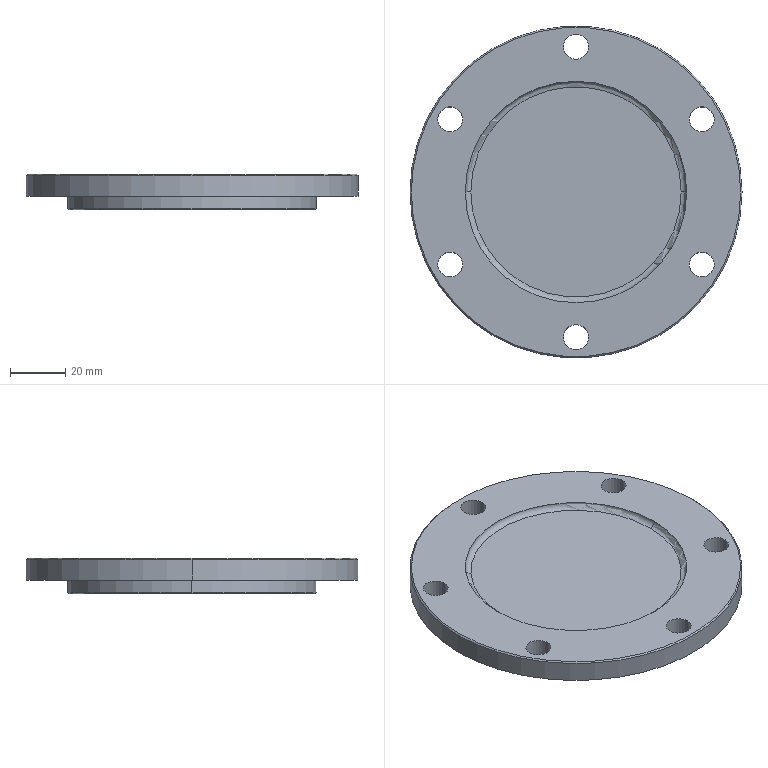Part | SolidWorks | features ICE 2, Chamfer 1, Extrusion 1, Fillet 1 | 1 solid | 29 faces | box 120 x 120 x 13 mm | volume 84178 mm3 | cylinder 18 | plane 5 | cone 4 | torus 2 | commonest cylinder face diameters 9 x12 80 x2 90 x2 120 x2
STEP:
#1=CARTESIAN_POINT('',(-38.,0.,6.));
#2=VERTEX_POINT('',#1);
#3=CARTESIAN_POINT('',(38.,0.,6.));
#4=VERTEX_POINT('',#3);
#5=CARTESIAN_POINT('',(0.,0.,6.));
#6=DIRECTION('',(0.,0.,1.));
#7=DIRECTION('',(1.,0.,0.));
#8=AXIS2_PLACEMENT_3D('',#5,#6,#7);
#9=CIRCLE('',#8,38.);
#10=EDGE_CURVE('',#2,#4,#9,.T.);
#11=ORIENTED_EDGE('',*,*,#10,.F.);
#12=CARTESIAN_POINT('',(-40.,0.,8.));
#13=VERTEX_POINT('',#12);
#14=CARTESIAN_POINT('',(-38.,0.,8.));
#15=DIRECTION('',(0.,1.,0.));
#16=DIRECTION('',(-1.,0.,0.));
#17=AXIS2_PLACEMENT_3D('',#14,#15,#16);
#18=CIRCLE('',#17,2.);
#19=EDGE_CURVE('',#2,#13,#18,.T.);
#20=ORIENTED_EDGE('',*,*,#19,.T.);
#21=CARTESIAN_POINT('',(40.,0.,8.));
#22=VERTEX_POINT('',#21);
#23=CARTESIAN_POINT('',(0.,0.,8.));
#24=DIRECTION('',(0.,0.,1.));
#25=DIRECTION('',(1.,0.,0.));
#26=AXIS2_PLACEMENT_3D('',#23,#24,#25);
#27=CIRCLE('',#26,40.);
#28=EDGE_CURVE('',#13,#22,#27,.T.);
#29=ORIENTED_EDGE('',*,*,#28,.T.);
#30=CARTESIAN_POINT('',(38.,0.,8.));
#31=DIRECTION('',(0.,-1.,0.));
#32=DIRECTION('',(0.,0.,-1.));
#33=AXIS2_PLACEMENT_3D('',#30,#31,#32);
#34=CIRCLE('',#33,2.);
#35=EDGE_CURVE('',#4,#22,#34,.T.);
#36=ORIENTED_EDGE('',*,*,#35,.F.);
#37=EDGE_LOOP('',(#11,#20,#29,#36));
#38=FACE_OUTER_BOUND('',#37,.T.);
#39=CARTESIAN_POINT('',(0.,0.,8.));
#40=DIRECTION('',(0.,0.,1.));
#41=DIRECTION('',(1.,0.,0.));
#42=AXIS2_PLACEMENT_3D('',#39,#40,#41);
#43=TOROIDAL_SURFACE('',#42,38.,2.);
#44=ADVANCED_FACE('',(#38),#43,.F.);
#45=CARTESIAN_POINT('',(59.5,0.,8.));
#46=VERTEX_POINT('',#45);
#47=CARTESIAN_POINT('',(-59.5,0.,8.));
#48=VERTEX_POINT('',#47);
#49=CARTESIAN_POINT('',(0.,0.,8.));
#50=DIRECTION('',(0.,0.,1.));
#51=DIRECTION('',(1.,0.,0.));
#52=AXIS2_PLACEMENT_3D('',#49,#50,#51);
#53=CIRCLE('',#52,59.5);
#54=EDGE_CURVE('',#46,#48,#53,.T.);
#55=ORIENTED_EDGE('',*,*,#54,.F.);
#56=CARTESIAN_POINT('',(60.,0.,7.5));
#57=VERTEX_POINT('',#56);
#58=CARTESIAN_POINT('',(59.5,0.,8.));
#59=DIRECTION('',(0.7071,0.,-0.7071));
#60=VECTOR('',#59,1000.);
#61=LINE('',#58,#60);
#62=EDGE_CURVE('',#46,#57,#61,.T.);
#63=ORIENTED_EDGE('',*,*,#62,.T.);
#64=CARTESIAN_POINT('',(-60.,0.,7.5));
#65=VERTEX_POINT('',#64);
#66=CARTESIAN_POINT('',(0.,0.,7.5));
#67=DIRECTION('',(0.,0.,-1.));
#68=DIRECTION('',(1.,0.,0.));
#69=AXIS2_PLACEMENT_3D('',#66,#67,#68);
#70=CIRCLE('',#69,60.);
#71=EDGE_CURVE('',#65,#57,#70,.T.);
#72=ORIENTED_EDGE('',*,*,#71,.F.);
#73=CARTESIAN_POINT('',(-59.5,0.,8.));
#74=DIRECTION('',(-0.7071,0.,-0.7071));
#75=VECTOR('',#74,1000.);
#76=LINE('',#73,#75);
#77=EDGE_CURVE('',#48,#65,#76,.T.);
#78=ORIENTED_EDGE('',*,*,#77,.F.);
#79=EDGE_LOOP('',(#55,#63,#72,#78));
#80=FACE_OUTER_BOUND('',#79,.T.);
#81=CARTESIAN_POINT('',(0.,0.,8.));
#82=DIRECTION('',(0.,0.,-1.));
#83=DIRECTION('',(-1.,0.,0.));
#84=AXIS2_PLACEMENT_3D('',#81,#82,#83);
#85=CONICAL_SURFACE('',#84,59.5,0.7854);
#86=ADVANCED_FACE('',(#80),#85,.T.);
#87=CARTESIAN_POINT('',(-44.5,0.,-5.));
#88=VERTEX_POINT('',#87);
#89=CARTESIAN_POINT('',(44.5,0.,-5.));
#90=VERTEX_POINT('',#89);
#91=CARTESIAN_POINT('',(0.,0.,-5.));
#92=DIRECTION('',(0.,0.,-1.));
#93=DIRECTION('',(-1.,0.,0.));
#94=AXIS2_PLACEMENT_3D('',#91,#92,#93);
#95=CIRCLE('',#94,44.5);
#96=EDGE_CURVE('',#88,#90,#95,.T.);
#97=ORIENTED_EDGE('',*,*,#96,.F.);
#98=CARTESIAN_POINT('',(-45.,0.,-4.5));
#99=VERTEX_POINT('',#98);
#100=CARTESIAN_POINT('',(-44.5,0.,-5.));
#101=DIRECTION('',(-0.7071,0.,0.7071));
#102=VECTOR('',#101,1000.);
#103=LINE('',#100,#102);
#104=EDGE_CURVE('',#88,#99,#103,.T.);
#105=ORIENTED_EDGE('',*,*,#104,.T.);
#106=CARTESIAN_POINT('',(45.,0.,-4.5));
#107=VERTEX_POINT('',#106);
#108=CARTESIAN_POINT('',(0.,0.,-4.5));
#109=DIRECTION('',(0.,0.,1.));
#110=DIRECTION('',(-1.,0.,0.));
#111=AXIS2_PLACEMENT_3D('',#108,#109,#110);
#112=CIRCLE('',#111,45.);
#113=EDGE_CURVE('',#107,#99,#112,.T.);
#114=ORIENTED_EDGE('',*,*,#113,.F.);
#115=CARTESIAN_POINT('',(44.5,0.,-5.));
#116=DIRECTION('',(0.7071,0.,0.7071));
#117=VECTOR('',#116,1000.);
#118=LINE('',#115,#117);
#119=EDGE_CURVE('',#90,#107,#118,.T.);
#120=ORIENTED_EDGE('',*,*,#119,.F.);
#121=EDGE_LOOP('',(#97,#105,#114,#120));
#122=FACE_OUTER_BOUND('',#121,.T.);
#123=CARTESIAN_POINT('',(0.,0.,-5.));
#124=DIRECTION('',(0.,0.,1.));
#125=DIRECTION('',(1.,0.,0.));
#126=AXIS2_PLACEMENT_3D('',#123,#124,#125);
#127=CONICAL_SURFACE('',#126,44.5,0.7854);
#128=ADVANCED_FACE('',(#122),#127,.T.);
#129=CARTESIAN_POINT('',(40.,0.,-5.));
#130=VERTEX_POINT('',#129);
#131=CARTESIAN_POINT('',(-40.,0.,-5.));
#132=VERTEX_POINT('',#131);
#133=CARTESIAN_POINT('',(0.,0.,-5.));
#134=DIRECTION('',(0.,0.,-1.));
#135=DIRECTION('',(-1.,0.,0.));
#136=AXIS2_PLACEMENT_3D('',#133,#134,#135);
#137=CIRCLE('',#136,40.);
#138=EDGE_CURVE('',#130,#132,#137,.T.);
#139=ORIENTED_EDGE('',*,*,#138,.T.);
#140=CARTESIAN_POINT('',(-40.,0.,0.));
#141=VERTEX_POINT('',#140);
#142=CARTESIAN_POINT('',(-40.,0.,-5.));
#143=DIRECTION('',(0.,0.,1.));
#144=VECTOR('',#143,1000.);
#145=LINE('',#142,#144);
#146=EDGE_CURVE('',#132,#141,#145,.T.);
#147=ORIENTED_EDGE('',*,*,#146,.T.);
#148=CARTESIAN_POINT('',(40.,0.,0.));
#149=VERTEX_POINT('',#148);
#150=CARTESIAN_POINT('',(0.,0.,0.));
#151=DIRECTION('',(0.,0.,-1.));
#152=DIRECTION('',(-1.,0.,0.));
#153=AXIS2_PLACEMENT_3D('',#150,#151,#152);
#154=CIRCLE('',#153,40.);
#155=EDGE_CURVE('',#149,#141,#154,.T.);
#156=ORIENTED_EDGE('',*,*,#155,.F.);
#157=CARTESIAN_POINT('',(40.,0.,-5.));
#158=DIRECTION('',(0.,0.,1.));
#159=VECTOR('',#158,1000.);
#160=LINE('',#157,#159);
#161=EDGE_CURVE('',#130,#149,#160,.T.);
#162=ORIENTED_EDGE('',*,*,#161,.F.);
#163=EDGE_LOOP('',(#139,#147,#156,#162));
#164=FACE_OUTER_BOUND('',#163,.T.);
#165=CARTESIAN_POINT('',(0.,0.,-5.));
#166=DIRECTION('',(0.,0.,1.));
#167=DIRECTION('',(1.,0.,0.));
#168=AXIS2_PLACEMENT_3D('',#165,#166,#167);
#169=CYLINDRICAL_SURFACE('',#168,40.);
#170=ADVANCED_FACE('',(#164),#169,.F.);
#171=ORIENTED_EDGE('',*,*,#113,.T.);
#172=CARTESIAN_POINT('',(-45.,0.,0.));
#173=VERTEX_POINT('',#172);
#174=CARTESIAN_POINT('',(-45.,0.,-5.));
#175=DIRECTION('',(0.,0.,1.));
#176=VECTOR('',#175,1000.);
#177=LINE('',#174,#176);
#178=EDGE_CURVE('',#99,#173,#177,.T.);
#179=ORIENTED_EDGE('',*,*,#178,.T.);
#180=CARTESIAN_POINT('',(45.,0.,0.));
#181=VERTEX_POINT('',#180);
#182=CARTESIAN_POINT('',(0.,0.,0.));
#183=DIRECTION('',(0.,0.,-1.));
#184=DIRECTION('',(1.,0.,0.));
#185=AXIS2_PLACEMENT_3D('',#182,#183,#184);
#186=CIRCLE('',#185,45.);
#187=EDGE_CURVE('',#173,#181,#186,.T.);
#188=ORIENTED_EDGE('',*,*,#187,.T.);
#189=CARTESIAN_POINT('',(45.,0.,-5.));
#190=DIRECTION('',(0.,0.,1.));
#191=VECTOR('',#190,1000.);
#192=LINE('',#189,#191);
#193=EDGE_CURVE('',#107,#181,#192,.T.);
#194=ORIENTED_EDGE('',*,*,#193,.F.);
#195=EDGE_LOOP('',(#171,#179,#188,#194));
#196=FACE_OUTER_BOUND('',#195,.T.);
#197=CARTESIAN_POINT('',(0.,0.,-5.));
#198=DIRECTION('',(0.,0.,1.));
#199=DIRECTION('',(1.,0.,0.));
#200=AXIS2_PLACEMENT_3D('',#197,#198,#199);
#201=CYLINDRICAL_SURFACE('',#200,45.);
#202=ADVANCED_FACE('',(#196),#201,.T.);
#203=CARTESIAN_POINT('',(-49.966,26.25,8.));
#204=VERTEX_POINT('',#203);
#205=CARTESIAN_POINT('',(-40.966,26.25,8.));
#206=VERTEX_POINT('',#205);
#207=CARTESIAN_POINT('',(-45.466,26.25,8.));
#208=DIRECTION('',(0.,0.,1.));
#209=DIRECTION('',(1.,0.,0.));
#210=AXIS2_PLACEMENT_3D('',#207,#208,#209);
#211=CIRCLE('',#210,4.5);
#212=EDGE_CURVE('',#204,#206,#211,.T.);
#213=ORIENTED_EDGE('',*,*,#212,.T.);
#214=CARTESIAN_POINT('',(-40.966,26.25,0.));
#215=VERTEX_POINT('',#214);
#216=CARTESIAN_POINT('',(-40.966,26.25,8.));
#217=DIRECTION('',(0.,0.,-1.));
#218=VECTOR('',#217,1000.);
#219=LINE('',#216,#218);
#220=EDGE_CURVE('',#206,#215,#219,.T.);
#221=ORIENTED_EDGE('',*,*,#220,.T.);
#222=CARTESIAN_POINT('',(-49.966,26.25,0.));
#223=VERTEX_POINT('',#222);
#224=CARTESIAN_POINT('',(-45.466,26.25,0.));
#225=DIRECTION('',(0.,0.,1.));
#226=DIRECTION('',(1.,0.,0.));
#227=AXIS2_PLACEMENT_3D('',#224,#225,#226);
#228=CIRCLE('',#227,4.5);
#229=EDGE_CURVE('',#223,#215,#228,.T.);
#230=ORIENTED_EDGE('',*,*,#229,.F.);
#231=CARTESIAN_POINT('',(-49.966,26.25,8.));
#232=DIRECTION('',(0.,0.,-1.));
#233=VECTOR('',#232,1000.);
#234=LINE('',#231,#233);
#235=EDGE_CURVE('',#204,#223,#234,.T.);
#236=ORIENTED_EDGE('',*,*,#235,.F.);
#237=EDGE_LOOP('',(#213,#221,#230,#236));
#238=FACE_OUTER_BOUND('',#237,.T.);
#239=CARTESIAN_POINT('',(-45.466,26.25,8.));
#240=DIRECTION('',(0.,0.,-1.));
#241=DIRECTION('',(-1.,0.,0.));
#242=AXIS2_PLACEMENT_3D('',#239,#240,#241);
#243=CYLINDRICAL_SURFACE('',#242,4.5);
#244=ADVANCED_FACE('',(#238),#243,.F.);
#245=CARTESIAN_POINT('',(-49.966,-26.25,8.));
#246=VERTEX_POINT('',#245);
#247=CARTESIAN_POINT('',(-40.966,-26.25,8.));
#248=VERTEX_POINT('',#247);
#249=CARTESIAN_POINT('',(-45.466,-26.25,8.));
#250=DIRECTION('',(0.,0.,1.));
#251=DIRECTION('',(1.,0.,0.));
#252=AXIS2_PLACEMENT_3D('',#249,#250,#251);
#253=CIRCLE('',#252,4.5);
#254=EDGE_CURVE('',#246,#248,#253,.T.);
#255=ORIENTED_EDGE('',*,*,#254,.T.);
#256=CARTESIAN_POINT('',(-40.966,-26.25,0.));
#257=VERTEX_POINT('',#256);
#258=CARTESIAN_POINT('',(-40.966,-26.25,8.));
#259=DIRECTION('',(0.,0.,-1.));
#260=VECTOR('',#259,1000.);
#261=LINE('',#258,#260);
#262=EDGE_CURVE('',#248,#257,#261,.T.);
#263=ORIENTED_EDGE('',*,*,#262,.T.);
#264=CARTESIAN_POINT('',(-49.966,-26.25,0.));
#265=VERTEX_POINT('',#264);
#266=CARTESIAN_POINT('',(-45.466,-26.25,0.));
#267=DIRECTION('',(0.,0.,1.));
#268=DIRECTION('',(1.,0.,0.));
#269=AXIS2_PLACEMENT_3D('',#266,#267,#268);
#270=CIRCLE('',#269,4.5);
#271=EDGE_CURVE('',#265,#257,#270,.T.);
#272=ORIENTED_EDGE('',*,*,#271,.F.);
#273=CARTESIAN_POINT('',(-49.966,-26.25,8.));
#274=DIRECTION('',(0.,0.,-1.));
#275=VECTOR('',#274,1000.);
#276=LINE('',#273,#275);
#277=EDGE_CURVE('',#246,#265,#276,.T.);
#278=ORIENTED_EDGE('',*,*,#277,.F.);
#279=EDGE_LOOP('',(#255,#263,#272,#278));
#280=FACE_OUTER_BOUND('',#279,.T.);
#281=CARTESIAN_POINT('',(-45.466,-26.25,8.));
#282=DIRECTION('',(0.,0.,-1.));
#283=DIRECTION('',(-1.,0.,0.));
#284=AXIS2_PLACEMENT_3D('',#281,#282,#283);
#285=CYLINDRICAL_SURFACE('',#284,4.5);
#286=ADVANCED_FACE('',(#280),#285,.F.);
#287=CARTESIAN_POINT('',(-4.5,-52.5,8.));
#288=VERTEX_POINT('',#287);
#289=CARTESIAN_POINT('',(4.5,-52.5,8.));
#290=VERTEX_POINT('',#289);
#291=CARTESIAN_POINT('',(0.,-52.5,8.));
#292=DIRECTION('',(0.,0.,1.));
#293=DIRECTION('',(1.,0.,0.));
#294=AXIS2_PLACEMENT_3D('',#291,#292,#293);
#295=CIRCLE('',#294,4.5);
#296=EDGE_CURVE('',#288,#290,#295,.T.);
#297=ORIENTED_EDGE('',*,*,#296,.T.);
#298=CARTESIAN_POINT('',(4.5,-52.5,0.));
#299=VERTEX_POINT('',#298);
#300=CARTESIAN_POINT('',(4.5,-52.5,8.));
#301=DIRECTION('',(0.,0.,-1.));
#302=VECTOR('',#301,1000.);
#303=LINE('',#300,#302);
#304=EDGE_CURVE('',#290,#299,#303,.T.);
#305=ORIENTED_EDGE('',*,*,#304,.T.);
#306=CARTESIAN_POINT('',(-4.5,-52.5,0.));
#307=VERTEX_POINT('',#306);
#308=CARTESIAN_POINT('',(0.,-52.5,0.));
#309=DIRECTION('',(0.,0.,1.));
#310=DIRECTION('',(1.,0.,0.));
#311=AXIS2_PLACEMENT_3D('',#308,#309,#310);
#312=CIRCLE('',#311,4.5);
#313=EDGE_CURVE('',#307,#299,#312,.T.);
#314=ORIENTED_EDGE('',*,*,#313,.F.);
#315=CARTESIAN_POINT('',(-4.5,-52.5,8.));
#316=DIRECTION('',(0.,0.,-1.));
#317=VECTOR('',#316,1000.);
#318=LINE('',#315,#317);
#319=EDGE_CURVE('',#288,#307,#318,.T.);
#320=ORIENTED_EDGE('',*,*,#319,.F.);
#321=EDGE_LOOP('',(#297,#305,#314,#320));
#322=FACE_OUTER_BOUND('',#321,.T.);
#323=CARTESIAN_POINT('',(0.,-52.5,8.));
#324=DIRECTION('',(0.,0.,-1.));
#325=DIRECTION('',(-1.,0.,0.));
#326=AXIS2_PLACEMENT_3D('',#323,#324,#325);
#327=CYLINDRICAL_SURFACE('',#326,4.5);
#328=ADVANCED_FACE('',(#322),#327,.F.);
#329=CARTESIAN_POINT('',(40.966,-26.25,8.));
#330=VERTEX_POINT('',#329);
#331=CARTESIAN_POINT('',(49.966,-26.25,8.));
#332=VERTEX_POINT('',#331);
#333=CARTESIAN_POINT('',(45.466,-26.25,8.));
#334=DIRECTION('',(0.,0.,1.));
#335=DIRECTION('',(1.,0.,0.));
#336=AXIS2_PLACEMENT_3D('',#333,#334,#335);
#337=CIRCLE('',#336,4.5);
#338=EDGE_CURVE('',#330,#332,#337,.T.);
#339=ORIENTED_EDGE('',*,*,#338,.T.);
#340=CARTESIAN_POINT('',(49.966,-26.25,0.));
#341=VERTEX_POINT('',#340);
#342=CARTESIAN_POINT('',(49.966,-26.25,8.));
#343=DIRECTION('',(0.,0.,-1.));
#344=VECTOR('',#343,1000.);
#345=LINE('',#342,#344);
#346=EDGE_CURVE('',#332,#341,#345,.T.);
#347=ORIENTED_EDGE('',*,*,#346,.T.);
#348=CARTESIAN_POINT('',(40.966,-26.25,0.));
#349=VERTEX_POINT('',#348);
#350=CARTESIAN_POINT('',(45.466,-26.25,0.));
#351=DIRECTION('',(0.,0.,1.));
#352=DIRECTION('',(1.,0.,0.));
#353=AXIS2_PLACEMENT_3D('',#350,#351,#352);
#354=CIRCLE('',#353,4.5);
#355=EDGE_CURVE('',#349,#341,#354,.T.);
#356=ORIENTED_EDGE('',*,*,#355,.F.);
#357=CARTESIAN_POINT('',(40.966,-26.25,8.));
#358=DIRECTION('',(0.,0.,-1.));
#359=VECTOR('',#358,1000.);
#360=LINE('',#357,#359);
#361=EDGE_CURVE('',#330,#349,#360,.T.);
#362=ORIENTED_EDGE('',*,*,#361,.F.);
#363=EDGE_LOOP('',(#339,#347,#356,#362));
#364=FACE_OUTER_BOUND('',#363,.T.);
#365=CARTESIAN_POINT('',(45.466,-26.25,8.));
#366=DIRECTION('',(0.,0.,-1.));
#367=DIRECTION('',(-1.,0.,0.));
#368=AXIS2_PLACEMENT_3D('',#365,#366,#367);
#369=CYLINDRICAL_SURFACE('',#368,4.5);
#370=ADVANCED_FACE('',(#364),#369,.F.);
#371=CARTESIAN_POINT('',(40.966,26.25,8.));
#372=VERTEX_POINT('',#371);
#373=CARTESIAN_POINT('',(49.966,26.25,8.));
#374=VERTEX_POINT('',#373);
#375=CARTESIAN_POINT('',(45.466,26.25,8.));
#376=DIRECTION('',(0.,0.,1.));
#377=DIRECTION('',(1.,0.,0.));
#378=AXIS2_PLACEMENT_3D('',#375,#376,#377);
#379=CIRCLE('',#378,4.5);
#380=EDGE_CURVE('',#372,#374,#379,.T.);
#381=ORIENTED_EDGE('',*,*,#380,.T.);
#382=CARTESIAN_POINT('',(49.966,26.25,0.));
#383=VERTEX_POINT('',#382);
#384=CARTESIAN_POINT('',(49.966,26.25,8.));
#385=DIRECTION('',(0.,0.,-1.));
#386=VECTOR('',#385,1000.);
#387=LINE('',#384,#386);
#388=EDGE_CURVE('',#374,#383,#387,.T.);
#389=ORIENTED_EDGE('',*,*,#388,.T.);
#390=CARTESIAN_POINT('',(40.966,26.25,0.));
#391=VERTEX_POINT('',#390);
#392=CARTESIAN_POINT('',(45.466,26.25,0.));
#393=DIRECTION('',(0.,0.,1.));
#394=DIRECTION('',(1.,0.,0.));
#395=AXIS2_PLACEMENT_3D('',#392,#393,#394);
#396=CIRCLE('',#395,4.5);
#397=EDGE_CURVE('',#391,#383,#396,.T.);
#398=ORIENTED_EDGE('',*,*,#397,.F.);
#399=CARTESIAN_POINT('',(40.966,26.25,8.));
#400=DIRECTION('',(0.,0.,-1.));
#401=VECTOR('',#400,1000.);
#402=LINE('',#399,#401);
#403=EDGE_CURVE('',#372,#391,#402,.T.);
#404=ORIENTED_EDGE('',*,*,#403,.F.);
#405=EDGE_LOOP('',(#381,#389,#398,#404));
#406=FACE_OUTER_BOUND('',#405,.T.);
#407=CARTESIAN_POINT('',(45.466,26.25,8.));
#408=DIRECTION('',(0.,0.,-1.));
#409=DIRECTION('',(-1.,0.,0.));
#410=AXIS2_PLACEMENT_3D('',#407,#408,#409);
#411=CYLINDRICAL_SURFACE('',#410,4.5);
#412=ADVANCED_FACE('',(#406),#411,.F.);
#413=CARTESIAN_POINT('',(-4.5,52.5,8.));
#414=VERTEX_POINT('',#413);
#415=CARTESIAN_POINT('',(4.5,52.5,8.));
#416=VERTEX_POINT('',#415);
#417=CARTESIAN_POINT('',(0.,52.5,8.));
#418=DIRECTION('',(0.,0.,1.));
#419=DIRECTION('',(1.,0.,0.));
#420=AXIS2_PLACEMENT_3D('',#417,#418,#419);
#421=CIRCLE('',#420,4.5);
#422=EDGE_CURVE('',#414,#416,#421,.T.);
#423=ORIENTED_EDGE('',*,*,#422,.T.);
#424=CARTESIAN_POINT('',(4.5,52.5,0.));
#425=VERTEX_POINT('',#424);
#426=CARTESIAN_POINT('',(4.5,52.5,8.));
#427=DIRECTION('',(0.,0.,-1.));
#428=VECTOR('',#427,1000.);
#429=LINE('',#426,#428);
#430=EDGE_CURVE('',#416,#425,#429,.T.);
#431=ORIENTED_EDGE('',*,*,#430,.T.);
#432=CARTESIAN_POINT('',(-4.5,52.5,0.));
#433=VERTEX_POINT('',#432);
#434=CARTESIAN_POINT('',(0.,52.5,0.));
#435=DIRECTION('',(0.,0.,1.));
#436=DIRECTION('',(1.,0.,0.));
#437=AXIS2_PLACEMENT_3D('',#434,#435,#436);
#438=CIRCLE('',#437,4.5);
#439=EDGE_CURVE('',#433,#425,#438,.T.);
#440=ORIENTED_EDGE('',*,*,#439,.F.);
#441=CARTESIAN_POINT('',(-4.5,52.5,8.));
#442=DIRECTION('',(0.,0.,-1.));
#443=VECTOR('',#442,1000.);
#444=LINE('',#441,#443);
#445=EDGE_CURVE('',#414,#433,#444,.T.);
#446=ORIENTED_EDGE('',*,*,#445,.F.);
#447=EDGE_LOOP('',(#423,#431,#440,#446));
#448=FACE_OUTER_BOUND('',#447,.T.);
#449=CARTESIAN_POINT('',(0.,52.5,8.));
#450=DIRECTION('',(0.,0.,-1.));
#451=DIRECTION('',(-1.,0.,0.));
#452=AXIS2_PLACEMENT_3D('',#449,#450,#451);
#453=CYLINDRICAL_SURFACE('',#452,4.5);
#454=ADVANCED_FACE('',(#448),#453,.F.);
#455=ORIENTED_EDGE('',*,*,#71,.T.);
#456=CARTESIAN_POINT('',(60.,0.,0.));
#457=VERTEX_POINT('',#456);
#458=CARTESIAN_POINT('',(60.,0.,8.));
#459=DIRECTION('',(0.,0.,-1.));
#460=VECTOR('',#459,1000.);
#461=LINE('',#458,#460);
#462=EDGE_CURVE('',#57,#457,#461,.T.);
#463=ORIENTED_EDGE('',*,*,#462,.T.);
#464=CARTESIAN_POINT('',(-60.,0.,0.));
#465=VERTEX_POINT('',#464);
#466=CARTESIAN_POINT('',(0.,0.,0.));
#467=DIRECTION('',(0.,0.,1.));
#468=DIRECTION('',(1.,0.,0.));
#469=AXIS2_PLACEMENT_3D('',#466,#467,#468);
#470=CIRCLE('',#469,60.);
#471=EDGE_CURVE('',#457,#465,#470,.T.);
#472=ORIENTED_EDGE('',*,*,#471,.T.);
#473=CARTESIAN_POINT('',(-60.,0.,8.));
#474=DIRECTION('',(0.,0.,-1.));
#475=VECTOR('',#474,1000.);
#476=LINE('',#473,#475);
#477=EDGE_CURVE('',#65,#465,#476,.T.);
#478=ORIENTED_EDGE('',*,*,#477,.F.);
#479=EDGE_LOOP('',(#455,#463,#472,#478));
#480=FACE_OUTER_BOUND('',#479,.T.);
#481=CARTESIAN_POINT('',(0.,0.,8.));
#482=DIRECTION('',(0.,0.,-1.));
#483=DIRECTION('',(-1.,0.,0.));
#484=AXIS2_PLACEMENT_3D('',#481,#482,#483);
#485=CYLINDRICAL_SURFACE('',#484,60.);
#486=ADVANCED_FACE('',(#480),#485,.T.);
#487=CARTESIAN_POINT('',(0.,0.,8.));
#488=DIRECTION('',(0.,0.,1.));
#489=DIRECTION('',(1.,0.,0.));
#490=AXIS2_PLACEMENT_3D('',#487,#488,#489);
#491=CIRCLE('',#490,40.);
#492=EDGE_CURVE('',#22,#13,#491,.T.);
#493=ORIENTED_EDGE('',*,*,#492,.F.);
#494=ORIENTED_EDGE('',*,*,#28,.F.);
#495=EDGE_LOOP('',(#493,#494));
#496=FACE_BOUND('',#495,.T.);
#497=CARTESIAN_POINT('',(0.,0.,8.));
#498=DIRECTION('',(0.,0.,1.));
#499=DIRECTION('',(1.,0.,0.));
#500=AXIS2_PLACEMENT_3D('',#497,#498,#499);
#501=CIRCLE('',#500,59.5);
#502=EDGE_CURVE('',#48,#46,#501,.T.);
#503=ORIENTED_EDGE('',*,*,#502,.T.);
#504=ORIENTED_EDGE('',*,*,#54,.T.);
#505=EDGE_LOOP('',(#503,#504));
#506=FACE_OUTER_BOUND('',#505,.T.);
#507=ORIENTED_EDGE('',*,*,#254,.F.);
#508=CARTESIAN_POINT('',(-45.466,-26.25,8.));
#509=DIRECTION('',(0.,0.,1.));
#510=DIRECTION('',(1.,0.,0.));
#511=AXIS2_PLACEMENT_3D('',#508,#509,#510);
#512=CIRCLE('',#511,4.5);
#513=EDGE_CURVE('',#248,#246,#512,.T.);
#514=ORIENTED_EDGE('',*,*,#513,.F.);
#515=EDGE_LOOP('',(#507,#514));
#516=FACE_BOUND('',#515,.T.);
#517=ORIENTED_EDGE('',*,*,#338,.F.);
#518=CARTESIAN_POINT('',(45.466,-26.25,8.));
#519=DIRECTION('',(0.,0.,1.));
#520=DIRECTION('',(1.,0.,0.));
#521=AXIS2_PLACEMENT_3D('',#518,#519,#520);
#522=CIRCLE('',#521,4.5);
#523=EDGE_CURVE('',#332,#330,#522,.T.);
#524=ORIENTED_EDGE('',*,*,#523,.F.);
#525=EDGE_LOOP('',(#517,#524));
#526=FACE_BOUND('',#525,.T.);
#527=ORIENTED_EDGE('',*,*,#422,.F.);
#528=CARTESIAN_POINT('',(0.,52.5,8.));
#529=DIRECTION('',(0.,0.,1.));
#530=DIRECTION('',(1.,0.,0.));
#531=AXIS2_PLACEMENT_3D('',#528,#529,#530);
#532=CIRCLE('',#531,4.5);
#533=EDGE_CURVE('',#416,#414,#532,.T.);
#534=ORIENTED_EDGE('',*,*,#533,.F.);
#535=EDGE_LOOP('',(#527,#534));
#536=FACE_BOUND('',#535,.T.);
#537=ORIENTED_EDGE('',*,*,#380,.F.);
#538=CARTESIAN_POINT('',(45.466,26.25,8.));
#539=DIRECTION('',(0.,0.,1.));
#540=DIRECTION('',(1.,0.,0.));
#541=AXIS2_PLACEMENT_3D('',#538,#539,#540);
#542=CIRCLE('',#541,4.5);
#543=EDGE_CURVE('',#374,#372,#542,.T.);
#544=ORIENTED_EDGE('',*,*,#543,.F.);
#545=EDGE_LOOP('',(#537,#544));
#546=FACE_BOUND('',#545,.T.);
#547=ORIENTED_EDGE('',*,*,#296,.F.);
#548=CARTESIAN_POINT('',(0.,-52.5,8.));
#549=DIRECTION('',(0.,0.,1.));
#550=DIRECTION('',(1.,0.,0.));
#551=AXIS2_PLACEMENT_3D('',#548,#549,#550);
#552=CIRCLE('',#551,4.5);
#553=EDGE_CURVE('',#290,#288,#552,.T.);
#554=ORIENTED_EDGE('',*,*,#553,.F.);
#555=EDGE_LOOP('',(#547,#554));
#556=FACE_BOUND('',#555,.T.);
#557=ORIENTED_EDGE('',*,*,#212,.F.);
#558=CARTESIAN_POINT('',(-45.466,26.25,8.));
#559=DIRECTION('',(0.,0.,1.));
#560=DIRECTION('',(1.,0.,0.));
#561=AXIS2_PLACEMENT_3D('',#558,#559,#560);
#562=CIRCLE('',#561,4.5);
#563=EDGE_CURVE('',#206,#204,#562,.T.);
#564=ORIENTED_EDGE('',*,*,#563,.F.);
#565=EDGE_LOOP('',(#557,#564));
#566=FACE_BOUND('',#565,.T.);
#567=CARTESIAN_POINT('',(0.,0.,8.));
#568=DIRECTION('',(0.,0.,1.));
#569=DIRECTION('',(1.,0.,0.));
#570=AXIS2_PLACEMENT_3D('',#567,#568,#569);
#571=PLANE('',#570);
#572=ADVANCED_FACE('',(#496,#506,#516,#526,#536,#546,#556,#566),#571,.T.);
#573=CARTESIAN_POINT('',(0.,0.,0.));
#574=DIRECTION('',(0.,0.,-1.));
#575=DIRECTION('',(1.,0.,0.));
#576=AXIS2_PLACEMENT_3D('',#573,#574,#575);
#577=CIRCLE('',#576,45.);
#578=EDGE_CURVE('',#181,#173,#577,.T.);
#579=ORIENTED_EDGE('',*,*,#578,.F.);
#580=ORIENTED_EDGE('',*,*,#187,.F.);
#581=EDGE_LOOP('',(#579,#580));
#582=FACE_BOUND('',#581,.T.);
#583=CARTESIAN_POINT('',(0.,0.,0.));
#584=DIRECTION('',(0.,0.,1.));
#585=DIRECTION('',(1.,0.,0.));
#586=AXIS2_PLACEMENT_3D('',#583,#584,#585);
#587=CIRCLE('',#586,60.);
#588=EDGE_CURVE('',#465,#457,#587,.T.);
#589=ORIENTED_EDGE('',*,*,#588,.F.);
#590=ORIENTED_EDGE('',*,*,#471,.F.);
#591=EDGE_LOOP('',(#589,#590));
#592=FACE_OUTER_BOUND('',#591,.T.);
#593=ORIENTED_EDGE('',*,*,#439,.T.);
#594=CARTESIAN_POINT('',(0.,52.5,0.));
#595=DIRECTION('',(0.,0.,1.));
#596=DIRECTION('',(1.,0.,0.));
#597=AXIS2_PLACEMENT_3D('',#594,#595,#596);
#598=CIRCLE('',#597,4.5);
#599=EDGE_CURVE('',#425,#433,#598,.T.);
#600=ORIENTED_EDGE('',*,*,#599,.T.);
#601=EDGE_LOOP('',(#593,#600));
#602=FACE_BOUND('',#601,.T.);
#603=ORIENTED_EDGE('',*,*,#397,.T.);
#604=CARTESIAN_POINT('',(45.466,26.25,0.));
#605=DIRECTION('',(0.,0.,1.));
#606=DIRECTION('',(1.,0.,0.));
#607=AXIS2_PLACEMENT_3D('',#604,#605,#606);
#608=CIRCLE('',#607,4.5);
#609=EDGE_CURVE('',#383,#391,#608,.T.);
#610=ORIENTED_EDGE('',*,*,#609,.T.);
#611=EDGE_LOOP('',(#603,#610));
#612=FACE_BOUND('',#611,.T.);
#613=ORIENTED_EDGE('',*,*,#355,.T.);
#614=CARTESIAN_POINT('',(45.466,-26.25,0.));
#615=DIRECTION('',(0.,0.,1.));
#616=DIRECTION('',(1.,0.,0.));
#617=AXIS2_PLACEMENT_3D('',#614,#615,#616);
#618=CIRCLE('',#617,4.5);
#619=EDGE_CURVE('',#341,#349,#618,.T.);
#620=ORIENTED_EDGE('',*,*,#619,.T.);
#621=EDGE_LOOP('',(#613,#620));
#622=FACE_BOUND('',#621,.T.);
#623=ORIENTED_EDGE('',*,*,#313,.T.);
#624=CARTESIAN_POINT('',(0.,-52.5,0.));
#625=DIRECTION('',(0.,0.,1.));
#626=DIRECTION('',(1.,0.,0.));
#627=AXIS2_PLACEMENT_3D('',#624,#625,#626);
#628=CIRCLE('',#627,4.5);
#629=EDGE_CURVE('',#299,#307,#628,.T.);
#630=ORIENTED_EDGE('',*,*,#629,.T.);
#631=EDGE_LOOP('',(#623,#630));
#632=FACE_BOUND('',#631,.T.);
#633=ORIENTED_EDGE('',*,*,#271,.T.);
#634=CARTESIAN_POINT('',(-45.466,-26.25,0.));
#635=DIRECTION('',(0.,0.,1.));
#636=DIRECTION('',(1.,0.,0.));
#637=AXIS2_PLACEMENT_3D('',#634,#635,#636);
#638=CIRCLE('',#637,4.5);
#639=EDGE_CURVE('',#257,#265,#638,.T.);
#640=ORIENTED_EDGE('',*,*,#639,.T.);
#641=EDGE_LOOP('',(#633,#640));
#642=FACE_BOUND('',#641,.T.);
#643=ORIENTED_EDGE('',*,*,#229,.T.);
#644=CARTESIAN_POINT('',(-45.466,26.25,0.));
#645=DIRECTION('',(0.,0.,1.));
#646=DIRECTION('',(1.,0.,0.));
#647=AXIS2_PLACEMENT_3D('',#644,#645,#646);
#648=CIRCLE('',#647,4.5);
#649=EDGE_CURVE('',#215,#223,#648,.T.);
#650=ORIENTED_EDGE('',*,*,#649,.T.);
#651=EDGE_LOOP('',(#643,#650));
#652=FACE_BOUND('',#651,.T.);
#653=CARTESIAN_POINT('',(0.,0.,0.));
#654=DIRECTION('',(0.,0.,1.));
#655=DIRECTION('',(1.,0.,0.));
#656=AXIS2_PLACEMENT_3D('',#653,#654,#655);
#657=PLANE('',#656);
#658=ADVANCED_FACE('',(#582,#592,#602,#612,#622,#632,#642,#652),#657,.F.);
#659=ORIENTED_EDGE('',*,*,#462,.F.);
#660=CARTESIAN_POINT('',(0.,0.,7.5));
#661=DIRECTION('',(0.,0.,-1.));
#662=DIRECTION('',(1.,0.,0.));
#663=AXIS2_PLACEMENT_3D('',#660,#661,#662);
#664=CIRCLE('',#663,60.);
#665=EDGE_CURVE('',#57,#65,#664,.T.);
#666=ORIENTED_EDGE('',*,*,#665,.T.);
#667=ORIENTED_EDGE('',*,*,#477,.T.);
#668=ORIENTED_EDGE('',*,*,#588,.T.);
#669=EDGE_LOOP('',(#659,#666,#667,#668));
#670=FACE_OUTER_BOUND('',#669,.T.);
#671=CARTESIAN_POINT('',(0.,0.,8.));
#672=DIRECTION('',(0.,0.,-1.));
#673=DIRECTION('',(-1.,0.,0.));
#674=AXIS2_PLACEMENT_3D('',#671,#672,#673);
#675=CYLINDRICAL_SURFACE('',#674,60.);
#676=ADVANCED_FACE('',(#670),#675,.T.);
#677=ORIENTED_EDGE('',*,*,#430,.F.);
#678=ORIENTED_EDGE('',*,*,#533,.T.);
#679=ORIENTED_EDGE('',*,*,#445,.T.);
#680=ORIENTED_EDGE('',*,*,#599,.F.);
#681=EDGE_LOOP('',(#677,#678,#679,#680));
#682=FACE_OUTER_BOUND('',#681,.T.);
#683=CARTESIAN_POINT('',(0.,52.5,8.));
#684=DIRECTION('',(0.,0.,-1.));
#685=DIRECTION('',(-1.,0.,0.));
#686=AXIS2_PLACEMENT_3D('',#683,#684,#685);
#687=CYLINDRICAL_SURFACE('',#686,4.5);
#688=ADVANCED_FACE('',(#682),#687,.F.);
#689=ORIENTED_EDGE('',*,*,#388,.F.);
#690=ORIENTED_EDGE('',*,*,#543,.T.);
#691=ORIENTED_EDGE('',*,*,#403,.T.);
#692=ORIENTED_EDGE('',*,*,#609,.F.);
#693=EDGE_LOOP('',(#689,#690,#691,#692));
#694=FACE_OUTER_BOUND('',#693,.T.);
#695=CARTESIAN_POINT('',(45.466,26.25,8.));
#696=DIRECTION('',(0.,0.,-1.));
#697=DIRECTION('',(-1.,0.,0.));
#698=AXIS2_PLACEMENT_3D('',#695,#696,#697);
#699=CYLINDRICAL_SURFACE('',#698,4.5);
#700=ADVANCED_FACE('',(#694),#699,.F.);
#701=ORIENTED_EDGE('',*,*,#346,.F.);
#702=ORIENTED_EDGE('',*,*,#523,.T.);
#703=ORIENTED_EDGE('',*,*,#361,.T.);
#704=ORIENTED_EDGE('',*,*,#619,.F.);
#705=EDGE_LOOP('',(#701,#702,#703,#704));
#706=FACE_OUTER_BOUND('',#705,.T.);
#707=CARTESIAN_POINT('',(45.466,-26.25,8.));
#708=DIRECTION('',(0.,0.,-1.));
#709=DIRECTION('',(-1.,0.,0.));
#710=AXIS2_PLACEMENT_3D('',#707,#708,#709);
#711=CYLINDRICAL_SURFACE('',#710,4.5);
#712=ADVANCED_FACE('',(#706),#711,.F.);
#713=ORIENTED_EDGE('',*,*,#304,.F.);
#714=ORIENTED_EDGE('',*,*,#553,.T.);
#715=ORIENTED_EDGE('',*,*,#319,.T.);
#716=ORIENTED_EDGE('',*,*,#629,.F.);
#717=EDGE_LOOP('',(#713,#714,#715,#716));
#718=FACE_OUTER_BOUND('',#717,.T.);
#719=CARTESIAN_POINT('',(0.,-52.5,8.));
#720=DIRECTION('',(0.,0.,-1.));
#721=DIRECTION('',(-1.,0.,0.));
#722=AXIS2_PLACEMENT_3D('',#719,#720,#721);
#723=CYLINDRICAL_SURFACE('',#722,4.5);
#724=ADVANCED_FACE('',(#718),#723,.F.);
#725=ORIENTED_EDGE('',*,*,#262,.F.);
#726=ORIENTED_EDGE('',*,*,#513,.T.);
#727=ORIENTED_EDGE('',*,*,#277,.T.);
#728=ORIENTED_EDGE('',*,*,#639,.F.);
#729=EDGE_LOOP('',(#725,#726,#727,#728));
#730=FACE_OUTER_BOUND('',#729,.T.);
#731=CARTESIAN_POINT('',(-45.466,-26.25,8.));
#732=DIRECTION('',(0.,0.,-1.));
#733=DIRECTION('',(-1.,0.,0.));
#734=AXIS2_PLACEMENT_3D('',#731,#732,#733);
#735=CYLINDRICAL_SURFACE('',#734,4.5);
#736=ADVANCED_FACE('',(#730),#735,.F.);
#737=ORIENTED_EDGE('',*,*,#220,.F.);
#738=ORIENTED_EDGE('',*,*,#563,.T.);
#739=ORIENTED_EDGE('',*,*,#235,.T.);
#740=ORIENTED_EDGE('',*,*,#649,.F.);
#741=EDGE_LOOP('',(#737,#738,#739,#740));
#742=FACE_OUTER_BOUND('',#741,.T.);
#743=CARTESIAN_POINT('',(-45.466,26.25,8.));
#744=DIRECTION('',(0.,0.,-1.));
#745=DIRECTION('',(-1.,0.,0.));
#746=AXIS2_PLACEMENT_3D('',#743,#744,#745);
#747=CYLINDRICAL_SURFACE('',#746,4.5);
#748=ADVANCED_FACE('',(#742),#747,.F.);
#749=CARTESIAN_POINT('',(0.,0.,-5.));
#750=DIRECTION('',(0.,0.,-1.));
#751=DIRECTION('',(-1.,0.,0.));
#752=AXIS2_PLACEMENT_3D('',#749,#750,#751);
#753=CIRCLE('',#752,44.5);
#754=EDGE_CURVE('',#90,#88,#753,.T.);
#755=ORIENTED_EDGE('',*,*,#754,.T.);
#756=ORIENTED_EDGE('',*,*,#96,.T.);
#757=EDGE_LOOP('',(#755,#756));
#758=FACE_OUTER_BOUND('',#757,.T.);
#759=ORIENTED_EDGE('',*,*,#138,.F.);
#760=CARTESIAN_POINT('',(0.,0.,-5.));
#761=DIRECTION('',(0.,0.,-1.));
#762=DIRECTION('',(-1.,0.,0.));
#763=AXIS2_PLACEMENT_3D('',#760,#761,#762);
#764=CIRCLE('',#763,40.);
#765=EDGE_CURVE('',#132,#130,#764,.T.);
#766=ORIENTED_EDGE('',*,*,#765,.F.);
#767=EDGE_LOOP('',(#759,#766));
#768=FACE_BOUND('',#767,.T.);
#769=CARTESIAN_POINT('',(0.,0.,-5.));
#770=DIRECTION('',(0.,0.,-1.));
#771=DIRECTION('',(-1.,0.,0.));
#772=AXIS2_PLACEMENT_3D('',#769,#770,#771);
#773=PLANE('',#772);
#774=ADVANCED_FACE('',(#758,#768),#773,.T.);
#775=ORIENTED_EDGE('',*,*,#178,.F.);
#776=CARTESIAN_POINT('',(0.,0.,-4.5));
#777=DIRECTION('',(0.,0.,1.));
#778=DIRECTION('',(-1.,0.,0.));
#779=AXIS2_PLACEMENT_3D('',#776,#777,#778);
#780=CIRCLE('',#779,45.);
#781=EDGE_CURVE('',#99,#107,#780,.T.);
#782=ORIENTED_EDGE('',*,*,#781,.T.);
#783=ORIENTED_EDGE('',*,*,#193,.T.);
#784=ORIENTED_EDGE('',*,*,#578,.T.);
#785=EDGE_LOOP('',(#775,#782,#783,#784));
#786=FACE_OUTER_BOUND('',#785,.T.);
#787=CARTESIAN_POINT('',(0.,0.,-5.));
#788=DIRECTION('',(0.,0.,1.));
#789=DIRECTION('',(1.,0.,0.));
#790=AXIS2_PLACEMENT_3D('',#787,#788,#789);
#791=CYLINDRICAL_SURFACE('',#790,45.);
#792=ADVANCED_FACE('',(#786),#791,.T.);
#793=ORIENTED_EDGE('',*,*,#146,.F.);
#794=ORIENTED_EDGE('',*,*,#765,.T.);
#795=ORIENTED_EDGE('',*,*,#161,.T.);
#796=CARTESIAN_POINT('',(0.,0.,0.));
#797=DIRECTION('',(0.,0.,-1.));
#798=DIRECTION('',(-1.,0.,0.));
#799=AXIS2_PLACEMENT_3D('',#796,#797,#798);
#800=CIRCLE('',#799,40.);
#801=EDGE_CURVE('',#141,#149,#800,.T.);
#802=ORIENTED_EDGE('',*,*,#801,.F.);
#803=EDGE_LOOP('',(#793,#794,#795,#802));
#804=FACE_OUTER_BOUND('',#803,.T.);
#805=CARTESIAN_POINT('',(0.,0.,-5.));
#806=DIRECTION('',(0.,0.,1.));
#807=DIRECTION('',(1.,0.,0.));
#808=AXIS2_PLACEMENT_3D('',#805,#806,#807);
#809=CYLINDRICAL_SURFACE('',#808,40.);
#810=ADVANCED_FACE('',(#804),#809,.F.);
#811=ORIENTED_EDGE('',*,*,#155,.T.);
#812=ORIENTED_EDGE('',*,*,#801,.T.);
#813=EDGE_LOOP('',(#811,#812));
#814=FACE_OUTER_BOUND('',#813,.T.);
#815=CARTESIAN_POINT('',(0.,0.,0.));
#816=DIRECTION('',(0.,0.,1.));
#817=DIRECTION('',(1.,0.,0.));
#818=AXIS2_PLACEMENT_3D('',#815,#816,#817);
#819=PLANE('',#818);
#820=ADVANCED_FACE('',(#814),#819,.F.);
#821=ORIENTED_EDGE('',*,*,#104,.F.);
#822=ORIENTED_EDGE('',*,*,#754,.F.);
#823=ORIENTED_EDGE('',*,*,#119,.T.);
#824=ORIENTED_EDGE('',*,*,#781,.F.);
#825=EDGE_LOOP('',(#821,#822,#823,#824));
#826=FACE_OUTER_BOUND('',#825,.T.);
#827=CARTESIAN_POINT('',(0.,0.,-5.));
#828=DIRECTION('',(0.,0.,1.));
#829=DIRECTION('',(1.,0.,0.));
#830=AXIS2_PLACEMENT_3D('',#827,#828,#829);
#831=CONICAL_SURFACE('',#830,44.5,0.7854);
#832=ADVANCED_FACE('',(#826),#831,.T.);
#833=ORIENTED_EDGE('',*,*,#62,.F.);
#834=ORIENTED_EDGE('',*,*,#502,.F.);
#835=ORIENTED_EDGE('',*,*,#77,.T.);
#836=ORIENTED_EDGE('',*,*,#665,.F.);
#837=EDGE_LOOP('',(#833,#834,#835,#836));
#838=FACE_OUTER_BOUND('',#837,.T.);
#839=CARTESIAN_POINT('',(0.,0.,8.));
#840=DIRECTION('',(0.,0.,-1.));
#841=DIRECTION('',(-1.,0.,0.));
#842=AXIS2_PLACEMENT_3D('',#839,#840,#841);
#843=CONICAL_SURFACE('',#842,59.5,0.7854);
#844=ADVANCED_FACE('',(#838),#843,.T.);
#845=CARTESIAN_POINT('',(0.,0.,6.));
#846=DIRECTION('',(0.,0.,1.));
#847=DIRECTION('',(1.,0.,0.));
#848=AXIS2_PLACEMENT_3D('',#845,#846,#847);
#849=CIRCLE('',#848,38.);
#850=EDGE_CURVE('',#4,#2,#849,.T.);
#851=ORIENTED_EDGE('',*,*,#850,.T.);
#852=ORIENTED_EDGE('',*,*,#10,.T.);
#853=EDGE_LOOP('',(#851,#852));
#854=FACE_OUTER_BOUND('',#853,.T.);
#855=CARTESIAN_POINT('',(0.,0.,6.));
#856=DIRECTION('',(0.,0.,1.));
#857=DIRECTION('',(1.,0.,0.));
#858=AXIS2_PLACEMENT_3D('',#855,#856,#857);
#859=PLANE('',#858);
#860=ADVANCED_FACE('',(#854),#859,.T.);
#861=ORIENTED_EDGE('',*,*,#19,.F.);
#862=ORIENTED_EDGE('',*,*,#850,.F.);
#863=ORIENTED_EDGE('',*,*,#35,.T.);
#864=ORIENTED_EDGE('',*,*,#492,.T.);
#865=EDGE_LOOP('',(#861,#862,#863,#864));
#866=FACE_OUTER_BOUND('',#865,.T.);
#867=CARTESIAN_POINT('',(0.,0.,8.));
#868=DIRECTION('',(0.,0.,1.));
#869=DIRECTION('',(1.,0.,0.));
#870=AXIS2_PLACEMENT_3D('',#867,#868,#869);
#871=TOROIDAL_SURFACE('',#870,38.,2.);
#872=ADVANCED_FACE('',(#866),#871,.F.);
#873=CLOSED_SHELL('',(#44,#86,#128,#170,#202,#244,#286,#328,#370,#412,#454,#486,#572,#658,#676,#688,#700,#712,#724,#736,#748,#774,#792,#810,#820,#832,#844,#860,#872));
#874=MANIFOLD_SOLID_BREP('',#873);
#875=CARTESIAN_POINT('',(0.,0.,0.));
#876=DIRECTION('',(0.,0.,1.));
#877=DIRECTION('',(1.,0.,0.));
#878=AXIS2_PLACEMENT_3D('',#875,#876,#877);
#879=(LENGTH_UNIT()NAMED_UNIT(*)SI_UNIT(.MILLI.,.METRE.));
#880=UNCERTAINTY_MEASURE_WITH_UNIT(LENGTH_MEASURE(0.00001),#879,'','');
#881=(NAMED_UNIT(*)PLANE_ANGLE_UNIT()SI_UNIT($,.RADIAN.));
#882=(NAMED_UNIT(*)SI_UNIT($,.STERADIAN.)SOLID_ANGLE_UNIT());
#883=(GEOMETRIC_REPRESENTATION_CONTEXT(3)GLOBAL_UNCERTAINTY_ASSIGNED_CONTEXT((#880))GLOBAL_UNIT_ASSIGNED_CONTEXT((#879,#881,#882))REPRESENTATION_CONTEXT('',''));
#884=ADVANCED_BREP_SHAPE_REPRESENTATION('',(#874,#878),#883);